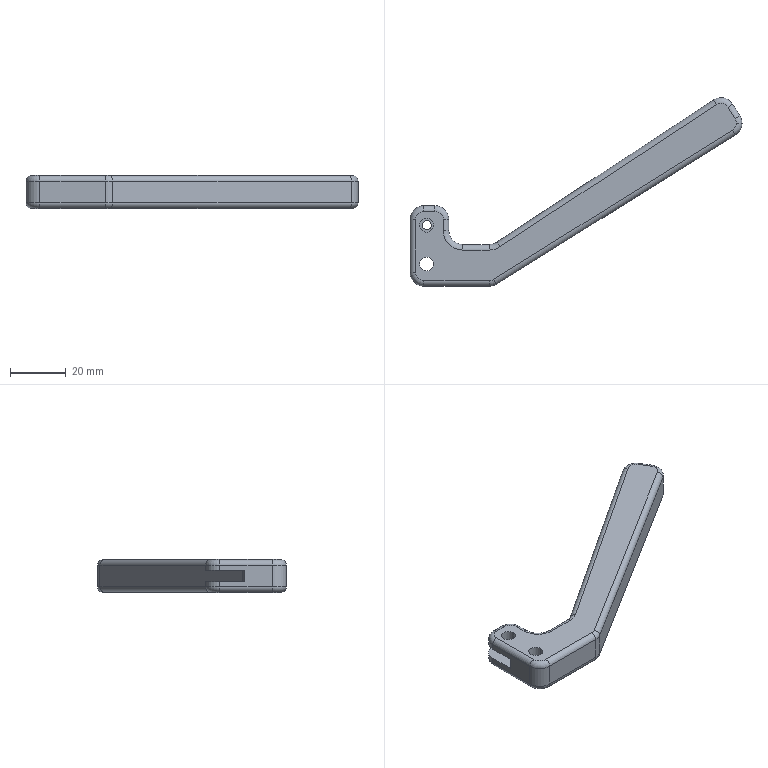Part | SolidWorks | features ICE 5, Attribute 3, Fillet 2, Extrusion 1 | 1 solid | 66 faces | box 119.634 x 67.923 x 11.9 mm | volume 22865 mm3 | cylinder 34 | torus 18 | plane 14 | commonest cylinder face diameters 4 x16 10 x12 5.05 x4 3.3 x2